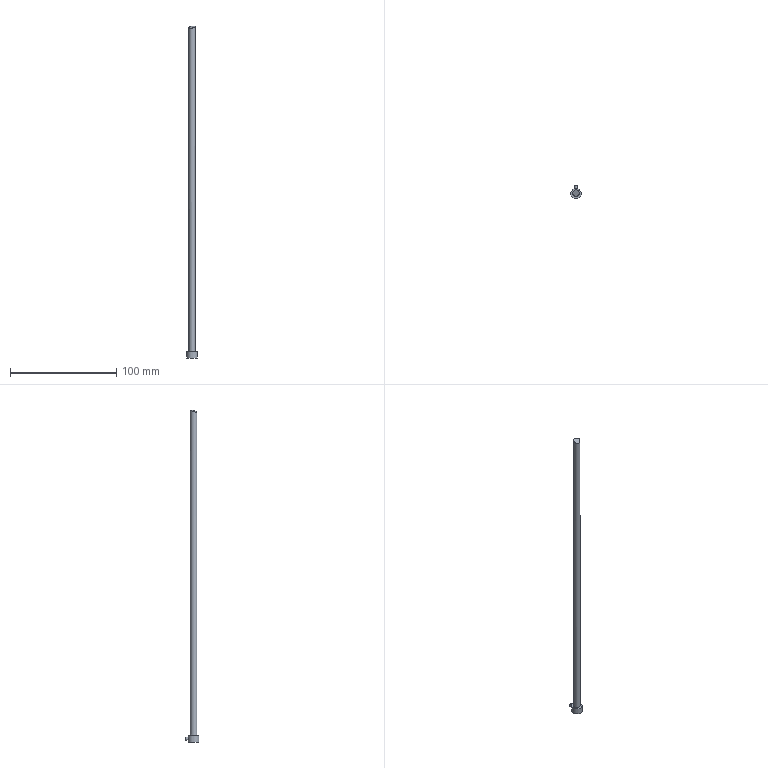Part | STEP file | E106-25-315 | 1 solid | 8 faces | box 10 x 13 x 312.463 mm | volume 9128 mm3 | cylinder 3 | plane 3 | spline 1 | cone 1 | commonest cylinder face diameters 3 x1 6 x1 10 x1